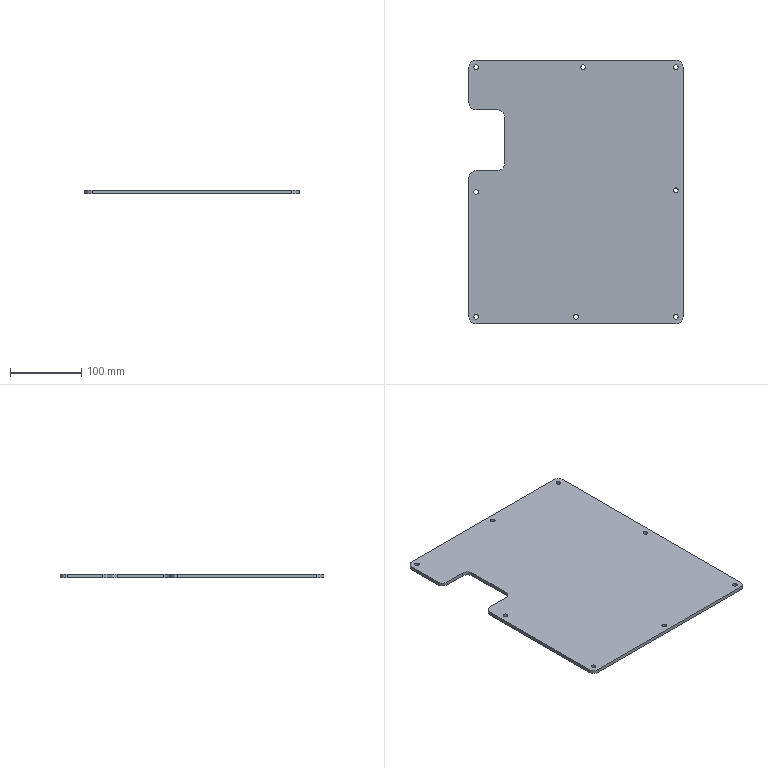Part | STEP file | 11-FG-01011 | 1 solid | 34 faces | box 300 x 370 x 5 mm | volume 531993 mm3 | cylinder 24 | plane 10 | commonest cylinder face diameters 6.5 x16 20 x8
STEP:
#1=CARTESIAN_POINT('',(-143.25,0.,0.));
#2=VERTEX_POINT('',#1);
#3=CARTESIAN_POINT('',(-136.75,0.,0.));
#4=VERTEX_POINT('',#3);
#5=CARTESIAN_POINT('',(-140.,0.,0.));
#6=DIRECTION('',(0.,0.,1.));
#7=DIRECTION('',(1.,0.,0.));
#8=AXIS2_PLACEMENT_3D('',#5,#6,#7);
#9=CIRCLE('',#8,3.25);
#10=EDGE_CURVE('',#2,#4,#9,.T.);
#11=ORIENTED_EDGE('',*,*,#10,.F.);
#12=CARTESIAN_POINT('',(-143.25,0.,5.));
#13=VERTEX_POINT('',#12);
#14=CARTESIAN_POINT('',(-143.25,0.,-5.));
#15=DIRECTION('',(0.,0.,1.));
#16=VECTOR('',#15,1000.);
#17=LINE('',#14,#16);
#18=EDGE_CURVE('',#2,#13,#17,.T.);
#19=ORIENTED_EDGE('',*,*,#18,.T.);
#20=CARTESIAN_POINT('',(-136.75,0.,5.));
#21=VERTEX_POINT('',#20);
#22=CARTESIAN_POINT('',(-140.,0.,5.));
#23=DIRECTION('',(0.,0.,1.));
#24=DIRECTION('',(1.,0.,0.));
#25=AXIS2_PLACEMENT_3D('',#22,#23,#24);
#26=CIRCLE('',#25,3.25);
#27=EDGE_CURVE('',#13,#21,#26,.T.);
#28=ORIENTED_EDGE('',*,*,#27,.T.);
#29=CARTESIAN_POINT('',(-136.75,0.,-5.));
#30=DIRECTION('',(0.,0.,1.));
#31=VECTOR('',#30,1000.);
#32=LINE('',#29,#31);
#33=EDGE_CURVE('',#4,#21,#32,.T.);
#34=ORIENTED_EDGE('',*,*,#33,.F.);
#35=EDGE_LOOP('',(#11,#19,#28,#34));
#36=FACE_OUTER_BOUND('',#35,.T.);
#37=CARTESIAN_POINT('',(-140.,0.,-5.));
#38=DIRECTION('',(0.,0.,1.));
#39=DIRECTION('',(1.,0.,0.));
#40=AXIS2_PLACEMENT_3D('',#37,#38,#39);
#41=CYLINDRICAL_SURFACE('',#40,3.25);
#42=ADVANCED_FACE('',(#36),#41,.F.);
#43=CARTESIAN_POINT('',(-143.25,-175.,0.));
#44=VERTEX_POINT('',#43);
#45=CARTESIAN_POINT('',(-136.75,-175.,0.));
#46=VERTEX_POINT('',#45);
#47=CARTESIAN_POINT('',(-140.,-175.,0.));
#48=DIRECTION('',(0.,0.,1.));
#49=DIRECTION('',(1.,0.,0.));
#50=AXIS2_PLACEMENT_3D('',#47,#48,#49);
#51=CIRCLE('',#50,3.25);
#52=EDGE_CURVE('',#44,#46,#51,.T.);
#53=ORIENTED_EDGE('',*,*,#52,.F.);
#54=CARTESIAN_POINT('',(-143.25,-175.,5.));
#55=VERTEX_POINT('',#54);
#56=CARTESIAN_POINT('',(-143.25,-175.,-5.));
#57=DIRECTION('',(0.,0.,1.));
#58=VECTOR('',#57,1000.);
#59=LINE('',#56,#58);
#60=EDGE_CURVE('',#44,#55,#59,.T.);
#61=ORIENTED_EDGE('',*,*,#60,.T.);
#62=CARTESIAN_POINT('',(-136.75,-175.,5.));
#63=VERTEX_POINT('',#62);
#64=CARTESIAN_POINT('',(-140.,-175.,5.));
#65=DIRECTION('',(0.,0.,1.));
#66=DIRECTION('',(1.,0.,0.));
#67=AXIS2_PLACEMENT_3D('',#64,#65,#66);
#68=CIRCLE('',#67,3.25);
#69=EDGE_CURVE('',#55,#63,#68,.T.);
#70=ORIENTED_EDGE('',*,*,#69,.T.);
#71=CARTESIAN_POINT('',(-136.75,-175.,-5.));
#72=DIRECTION('',(0.,0.,1.));
#73=VECTOR('',#72,1000.);
#74=LINE('',#71,#73);
#75=EDGE_CURVE('',#46,#63,#74,.T.);
#76=ORIENTED_EDGE('',*,*,#75,.F.);
#77=EDGE_LOOP('',(#53,#61,#70,#76));
#78=FACE_OUTER_BOUND('',#77,.T.);
#79=CARTESIAN_POINT('',(-140.,-175.,-5.));
#80=DIRECTION('',(0.,0.,1.));
#81=DIRECTION('',(1.,0.,0.));
#82=AXIS2_PLACEMENT_3D('',#79,#80,#81);
#83=CYLINDRICAL_SURFACE('',#82,3.25);
#84=ADVANCED_FACE('',(#78),#83,.F.);
#85=CARTESIAN_POINT('',(-3.25,-175.,0.));
#86=VERTEX_POINT('',#85);
#87=CARTESIAN_POINT('',(3.25,-175.,0.));
#88=VERTEX_POINT('',#87);
#89=CARTESIAN_POINT('',(0.,-175.,0.));
#90=DIRECTION('',(0.,0.,1.));
#91=DIRECTION('',(1.,0.,0.));
#92=AXIS2_PLACEMENT_3D('',#89,#90,#91);
#93=CIRCLE('',#92,3.25);
#94=EDGE_CURVE('',#86,#88,#93,.T.);
#95=ORIENTED_EDGE('',*,*,#94,.F.);
#96=CARTESIAN_POINT('',(-3.25,-175.,5.));
#97=VERTEX_POINT('',#96);
#98=CARTESIAN_POINT('',(-3.25,-175.,-5.));
#99=DIRECTION('',(0.,0.,1.));
#100=VECTOR('',#99,1000.);
#101=LINE('',#98,#100);
#102=EDGE_CURVE('',#86,#97,#101,.T.);
#103=ORIENTED_EDGE('',*,*,#102,.T.);
#104=CARTESIAN_POINT('',(3.25,-175.,5.));
#105=VERTEX_POINT('',#104);
#106=CARTESIAN_POINT('',(0.,-175.,5.));
#107=DIRECTION('',(0.,0.,1.));
#108=DIRECTION('',(1.,0.,0.));
#109=AXIS2_PLACEMENT_3D('',#106,#107,#108);
#110=CIRCLE('',#109,3.25);
#111=EDGE_CURVE('',#97,#105,#110,.T.);
#112=ORIENTED_EDGE('',*,*,#111,.T.);
#113=CARTESIAN_POINT('',(3.25,-175.,-5.));
#114=DIRECTION('',(0.,0.,1.));
#115=VECTOR('',#114,1000.);
#116=LINE('',#113,#115);
#117=EDGE_CURVE('',#88,#105,#116,.T.);
#118=ORIENTED_EDGE('',*,*,#117,.F.);
#119=EDGE_LOOP('',(#95,#103,#112,#118));
#120=FACE_OUTER_BOUND('',#119,.T.);
#121=CARTESIAN_POINT('',(0.,-175.,-5.));
#122=DIRECTION('',(0.,0.,1.));
#123=DIRECTION('',(1.,0.,0.));
#124=AXIS2_PLACEMENT_3D('',#121,#122,#123);
#125=CYLINDRICAL_SURFACE('',#124,3.25);
#126=ADVANCED_FACE('',(#120),#125,.F.);
#127=CARTESIAN_POINT('',(136.75,-175.,0.));
#128=VERTEX_POINT('',#127);
#129=CARTESIAN_POINT('',(143.25,-175.,0.));
#130=VERTEX_POINT('',#129);
#131=CARTESIAN_POINT('',(140.,-175.,0.));
#132=DIRECTION('',(0.,0.,1.));
#133=DIRECTION('',(1.,0.,0.));
#134=AXIS2_PLACEMENT_3D('',#131,#132,#133);
#135=CIRCLE('',#134,3.25);
#136=EDGE_CURVE('',#128,#130,#135,.T.);
#137=ORIENTED_EDGE('',*,*,#136,.F.);
#138=CARTESIAN_POINT('',(136.75,-175.,5.));
#139=VERTEX_POINT('',#138);
#140=CARTESIAN_POINT('',(136.75,-175.,-5.));
#141=DIRECTION('',(0.,0.,1.));
#142=VECTOR('',#141,1000.);
#143=LINE('',#140,#142);
#144=EDGE_CURVE('',#128,#139,#143,.T.);
#145=ORIENTED_EDGE('',*,*,#144,.T.);
#146=CARTESIAN_POINT('',(143.25,-175.,5.));
#147=VERTEX_POINT('',#146);
#148=CARTESIAN_POINT('',(140.,-175.,5.));
#149=DIRECTION('',(0.,0.,1.));
#150=DIRECTION('',(1.,0.,0.));
#151=AXIS2_PLACEMENT_3D('',#148,#149,#150);
#152=CIRCLE('',#151,3.25);
#153=EDGE_CURVE('',#139,#147,#152,.T.);
#154=ORIENTED_EDGE('',*,*,#153,.T.);
#155=CARTESIAN_POINT('',(143.25,-175.,-5.));
#156=DIRECTION('',(0.,0.,1.));
#157=VECTOR('',#156,1000.);
#158=LINE('',#155,#157);
#159=EDGE_CURVE('',#130,#147,#158,.T.);
#160=ORIENTED_EDGE('',*,*,#159,.F.);
#161=EDGE_LOOP('',(#137,#145,#154,#160));
#162=FACE_OUTER_BOUND('',#161,.T.);
#163=CARTESIAN_POINT('',(140.,-175.,-5.));
#164=DIRECTION('',(0.,0.,1.));
#165=DIRECTION('',(1.,0.,0.));
#166=AXIS2_PLACEMENT_3D('',#163,#164,#165);
#167=CYLINDRICAL_SURFACE('',#166,3.25);
#168=ADVANCED_FACE('',(#162),#167,.F.);
#169=CARTESIAN_POINT('',(136.75,2.5,0.));
#170=VERTEX_POINT('',#169);
#171=CARTESIAN_POINT('',(143.25,2.5,0.));
#172=VERTEX_POINT('',#171);
#173=CARTESIAN_POINT('',(140.,2.5,0.));
#174=DIRECTION('',(0.,0.,1.));
#175=DIRECTION('',(1.,0.,0.));
#176=AXIS2_PLACEMENT_3D('',#173,#174,#175);
#177=CIRCLE('',#176,3.25);
#178=EDGE_CURVE('',#170,#172,#177,.T.);
#179=ORIENTED_EDGE('',*,*,#178,.F.);
#180=CARTESIAN_POINT('',(136.75,2.5,5.));
#181=VERTEX_POINT('',#180);
#182=CARTESIAN_POINT('',(136.75,2.5,-5.));
#183=DIRECTION('',(0.,0.,1.));
#184=VECTOR('',#183,1000.);
#185=LINE('',#182,#184);
#186=EDGE_CURVE('',#170,#181,#185,.T.);
#187=ORIENTED_EDGE('',*,*,#186,.T.);
#188=CARTESIAN_POINT('',(143.25,2.5,5.));
#189=VERTEX_POINT('',#188);
#190=CARTESIAN_POINT('',(140.,2.5,5.));
#191=DIRECTION('',(0.,0.,1.));
#192=DIRECTION('',(1.,0.,0.));
#193=AXIS2_PLACEMENT_3D('',#190,#191,#192);
#194=CIRCLE('',#193,3.25);
#195=EDGE_CURVE('',#181,#189,#194,.T.);
#196=ORIENTED_EDGE('',*,*,#195,.T.);
#197=CARTESIAN_POINT('',(143.25,2.5,-5.));
#198=DIRECTION('',(0.,0.,1.));
#199=VECTOR('',#198,1000.);
#200=LINE('',#197,#199);
#201=EDGE_CURVE('',#172,#189,#200,.T.);
#202=ORIENTED_EDGE('',*,*,#201,.F.);
#203=EDGE_LOOP('',(#179,#187,#196,#202));
#204=FACE_OUTER_BOUND('',#203,.T.);
#205=CARTESIAN_POINT('',(140.,2.5,-5.));
#206=DIRECTION('',(0.,0.,1.));
#207=DIRECTION('',(1.,0.,0.));
#208=AXIS2_PLACEMENT_3D('',#205,#206,#207);
#209=CYLINDRICAL_SURFACE('',#208,3.25);
#210=ADVANCED_FACE('',(#204),#209,.F.);
#211=CARTESIAN_POINT('',(136.75,175.,0.));
#212=VERTEX_POINT('',#211);
#213=CARTESIAN_POINT('',(143.25,175.,0.));
#214=VERTEX_POINT('',#213);
#215=CARTESIAN_POINT('',(140.,175.,0.));
#216=DIRECTION('',(0.,0.,1.));
#217=DIRECTION('',(1.,0.,0.));
#218=AXIS2_PLACEMENT_3D('',#215,#216,#217);
#219=CIRCLE('',#218,3.25);
#220=EDGE_CURVE('',#212,#214,#219,.T.);
#221=ORIENTED_EDGE('',*,*,#220,.F.);
#222=CARTESIAN_POINT('',(136.75,175.,5.));
#223=VERTEX_POINT('',#222);
#224=CARTESIAN_POINT('',(136.75,175.,-5.));
#225=DIRECTION('',(0.,0.,1.));
#226=VECTOR('',#225,1000.);
#227=LINE('',#224,#226);
#228=EDGE_CURVE('',#212,#223,#227,.T.);
#229=ORIENTED_EDGE('',*,*,#228,.T.);
#230=CARTESIAN_POINT('',(143.25,175.,5.));
#231=VERTEX_POINT('',#230);
#232=CARTESIAN_POINT('',(140.,175.,5.));
#233=DIRECTION('',(0.,0.,1.));
#234=DIRECTION('',(1.,0.,0.));
#235=AXIS2_PLACEMENT_3D('',#232,#233,#234);
#236=CIRCLE('',#235,3.25);
#237=EDGE_CURVE('',#223,#231,#236,.T.);
#238=ORIENTED_EDGE('',*,*,#237,.T.);
#239=CARTESIAN_POINT('',(143.25,175.,-5.));
#240=DIRECTION('',(0.,0.,1.));
#241=VECTOR('',#240,1000.);
#242=LINE('',#239,#241);
#243=EDGE_CURVE('',#214,#231,#242,.T.);
#244=ORIENTED_EDGE('',*,*,#243,.F.);
#245=EDGE_LOOP('',(#221,#229,#238,#244));
#246=FACE_OUTER_BOUND('',#245,.T.);
#247=CARTESIAN_POINT('',(140.,175.,-5.));
#248=DIRECTION('',(0.,0.,1.));
#249=DIRECTION('',(1.,0.,0.));
#250=AXIS2_PLACEMENT_3D('',#247,#248,#249);
#251=CYLINDRICAL_SURFACE('',#250,3.25);
#252=ADVANCED_FACE('',(#246),#251,.F.);
#253=CARTESIAN_POINT('',(6.75,175.,0.));
#254=VERTEX_POINT('',#253);
#255=CARTESIAN_POINT('',(13.25,175.,0.));
#256=VERTEX_POINT('',#255);
#257=CARTESIAN_POINT('',(10.,175.,0.));
#258=DIRECTION('',(0.,0.,1.));
#259=DIRECTION('',(1.,0.,0.));
#260=AXIS2_PLACEMENT_3D('',#257,#258,#259);
#261=CIRCLE('',#260,3.25);
#262=EDGE_CURVE('',#254,#256,#261,.T.);
#263=ORIENTED_EDGE('',*,*,#262,.F.);
#264=CARTESIAN_POINT('',(6.75,175.,5.));
#265=VERTEX_POINT('',#264);
#266=CARTESIAN_POINT('',(6.75,175.,-5.));
#267=DIRECTION('',(0.,0.,1.));
#268=VECTOR('',#267,1000.);
#269=LINE('',#266,#268);
#270=EDGE_CURVE('',#254,#265,#269,.T.);
#271=ORIENTED_EDGE('',*,*,#270,.T.);
#272=CARTESIAN_POINT('',(13.25,175.,5.));
#273=VERTEX_POINT('',#272);
#274=CARTESIAN_POINT('',(10.,175.,5.));
#275=DIRECTION('',(0.,0.,1.));
#276=DIRECTION('',(1.,0.,0.));
#277=AXIS2_PLACEMENT_3D('',#274,#275,#276);
#278=CIRCLE('',#277,3.25);
#279=EDGE_CURVE('',#265,#273,#278,.T.);
#280=ORIENTED_EDGE('',*,*,#279,.T.);
#281=CARTESIAN_POINT('',(13.25,175.,-5.));
#282=DIRECTION('',(0.,0.,1.));
#283=VECTOR('',#282,1000.);
#284=LINE('',#281,#283);
#285=EDGE_CURVE('',#256,#273,#284,.T.);
#286=ORIENTED_EDGE('',*,*,#285,.F.);
#287=EDGE_LOOP('',(#263,#271,#280,#286));
#288=FACE_OUTER_BOUND('',#287,.T.);
#289=CARTESIAN_POINT('',(10.,175.,-5.));
#290=DIRECTION('',(0.,0.,1.));
#291=DIRECTION('',(1.,0.,0.));
#292=AXIS2_PLACEMENT_3D('',#289,#290,#291);
#293=CYLINDRICAL_SURFACE('',#292,3.25);
#294=ADVANCED_FACE('',(#288),#293,.F.);
#295=CARTESIAN_POINT('',(-143.25,175.,0.));
#296=VERTEX_POINT('',#295);
#297=CARTESIAN_POINT('',(-136.75,175.,0.));
#298=VERTEX_POINT('',#297);
#299=CARTESIAN_POINT('',(-140.,175.,0.));
#300=DIRECTION('',(0.,0.,1.));
#301=DIRECTION('',(1.,0.,0.));
#302=AXIS2_PLACEMENT_3D('',#299,#300,#301);
#303=CIRCLE('',#302,3.25);
#304=EDGE_CURVE('',#296,#298,#303,.T.);
#305=ORIENTED_EDGE('',*,*,#304,.F.);
#306=CARTESIAN_POINT('',(-143.25,175.,5.));
#307=VERTEX_POINT('',#306);
#308=CARTESIAN_POINT('',(-143.25,175.,-5.));
#309=DIRECTION('',(0.,0.,1.));
#310=VECTOR('',#309,1000.);
#311=LINE('',#308,#310);
#312=EDGE_CURVE('',#296,#307,#311,.T.);
#313=ORIENTED_EDGE('',*,*,#312,.T.);
#314=CARTESIAN_POINT('',(-136.75,175.,5.));
#315=VERTEX_POINT('',#314);
#316=CARTESIAN_POINT('',(-140.,175.,5.));
#317=DIRECTION('',(0.,0.,1.));
#318=DIRECTION('',(1.,0.,0.));
#319=AXIS2_PLACEMENT_3D('',#316,#317,#318);
#320=CIRCLE('',#319,3.25);
#321=EDGE_CURVE('',#307,#315,#320,.T.);
#322=ORIENTED_EDGE('',*,*,#321,.T.);
#323=CARTESIAN_POINT('',(-136.75,175.,-5.));
#324=DIRECTION('',(0.,0.,1.));
#325=VECTOR('',#324,1000.);
#326=LINE('',#323,#325);
#327=EDGE_CURVE('',#298,#315,#326,.T.);
#328=ORIENTED_EDGE('',*,*,#327,.F.);
#329=EDGE_LOOP('',(#305,#313,#322,#328));
#330=FACE_OUTER_BOUND('',#329,.T.);
#331=CARTESIAN_POINT('',(-140.,175.,-5.));
#332=DIRECTION('',(0.,0.,1.));
#333=DIRECTION('',(1.,0.,0.));
#334=AXIS2_PLACEMENT_3D('',#331,#332,#333);
#335=CYLINDRICAL_SURFACE('',#334,3.25);
#336=ADVANCED_FACE('',(#330),#335,.F.);
#337=CARTESIAN_POINT('',(-150.,175.,0.));
#338=VERTEX_POINT('',#337);
#339=CARTESIAN_POINT('',(-150.,125.,0.));
#340=VERTEX_POINT('',#339);
#341=CARTESIAN_POINT('',(-150.,185.,0.));
#342=DIRECTION('',(0.,-1.,0.));
#343=VECTOR('',#342,1000.);
#344=LINE('',#341,#343);
#345=EDGE_CURVE('',#338,#340,#344,.T.);
#346=ORIENTED_EDGE('',*,*,#345,.T.);
#347=CARTESIAN_POINT('',(-150.,125.,5.));
#348=VERTEX_POINT('',#347);
#349=CARTESIAN_POINT('',(-150.,125.,5.));
#350=DIRECTION('',(0.,0.,1.));
#351=VECTOR('',#350,1000.);
#352=LINE('',#349,#351);
#353=EDGE_CURVE('',#340,#348,#352,.T.);
#354=ORIENTED_EDGE('',*,*,#353,.T.);
#355=CARTESIAN_POINT('',(-150.,175.,5.));
#356=VERTEX_POINT('',#355);
#357=CARTESIAN_POINT('',(-150.,185.,5.));
#358=DIRECTION('',(0.,-1.,0.));
#359=VECTOR('',#358,1000.);
#360=LINE('',#357,#359);
#361=EDGE_CURVE('',#356,#348,#360,.T.);
#362=ORIENTED_EDGE('',*,*,#361,.F.);
#363=CARTESIAN_POINT('',(-150.,175.,5.));
#364=DIRECTION('',(0.,0.,-1.));
#365=VECTOR('',#364,1000.);
#366=LINE('',#363,#365);
#367=EDGE_CURVE('',#356,#338,#366,.T.);
#368=ORIENTED_EDGE('',*,*,#367,.T.);
#369=EDGE_LOOP('',(#346,#354,#362,#368));
#370=FACE_OUTER_BOUND('',#369,.T.);
#371=CARTESIAN_POINT('',(-150.,185.,5.));
#372=DIRECTION('',(1.,0.,0.));
#373=DIRECTION('',(0.,1.,0.));
#374=AXIS2_PLACEMENT_3D('',#371,#372,#373);
#375=PLANE('',#374);
#376=ADVANCED_FACE('',(#370),#375,.F.);
#377=CARTESIAN_POINT('',(150.,-175.,5.));
#378=VERTEX_POINT('',#377);
#379=CARTESIAN_POINT('',(150.,175.,5.));
#380=VERTEX_POINT('',#379);
#381=CARTESIAN_POINT('',(150.,185.,5.));
#382=DIRECTION('',(0.,1.,0.));
#383=VECTOR('',#382,1000.);
#384=LINE('',#381,#383);
#385=EDGE_CURVE('',#378,#380,#384,.T.);
#386=ORIENTED_EDGE('',*,*,#385,.F.);
#387=CARTESIAN_POINT('',(150.,-175.,0.));
#388=VERTEX_POINT('',#387);
#389=CARTESIAN_POINT('',(150.,-175.,5.));
#390=DIRECTION('',(0.,0.,-1.));
#391=VECTOR('',#390,1000.);
#392=LINE('',#389,#391);
#393=EDGE_CURVE('',#378,#388,#392,.T.);
#394=ORIENTED_EDGE('',*,*,#393,.T.);
#395=CARTESIAN_POINT('',(150.,175.,0.));
#396=VERTEX_POINT('',#395);
#397=CARTESIAN_POINT('',(150.,185.,0.));
#398=DIRECTION('',(0.,1.,0.));
#399=VECTOR('',#398,1000.);
#400=LINE('',#397,#399);
#401=EDGE_CURVE('',#388,#396,#400,.T.);
#402=ORIENTED_EDGE('',*,*,#401,.T.);
#403=CARTESIAN_POINT('',(150.,175.,5.));
#404=DIRECTION('',(0.,0.,1.));
#405=VECTOR('',#404,1000.);
#406=LINE('',#403,#405);
#407=EDGE_CURVE('',#396,#380,#406,.T.);
#408=ORIENTED_EDGE('',*,*,#407,.T.);
#409=EDGE_LOOP('',(#386,#394,#402,#408));
#410=FACE_OUTER_BOUND('',#409,.T.);
#411=CARTESIAN_POINT('',(150.,185.,5.));
#412=DIRECTION('',(-1.,0.,0.));
#413=DIRECTION('',(0.,-1.,0.));
#414=AXIS2_PLACEMENT_3D('',#411,#412,#413);
#415=PLANE('',#414);
#416=ADVANCED_FACE('',(#410),#415,.F.);
#417=CARTESIAN_POINT('',(140.,185.,5.));
#418=VERTEX_POINT('',#417);
#419=CARTESIAN_POINT('',(-140.,185.,5.));
#420=VERTEX_POINT('',#419);
#421=CARTESIAN_POINT('',(-150.,185.,5.));
#422=DIRECTION('',(-1.,0.,0.));
#423=VECTOR('',#422,1000.);
#424=LINE('',#421,#423);
#425=EDGE_CURVE('',#418,#420,#424,.T.);
#426=ORIENTED_EDGE('',*,*,#425,.F.);
#427=CARTESIAN_POINT('',(140.,185.,0.));
#428=VERTEX_POINT('',#427);
#429=CARTESIAN_POINT('',(140.,185.,5.));
#430=DIRECTION('',(0.,0.,-1.));
#431=VECTOR('',#430,1000.);
#432=LINE('',#429,#431);
#433=EDGE_CURVE('',#418,#428,#432,.T.);
#434=ORIENTED_EDGE('',*,*,#433,.T.);
#435=CARTESIAN_POINT('',(-140.,185.,0.));
#436=VERTEX_POINT('',#435);
#437=CARTESIAN_POINT('',(-150.,185.,0.));
#438=DIRECTION('',(-1.,0.,0.));
#439=VECTOR('',#438,1000.);
#440=LINE('',#437,#439);
#441=EDGE_CURVE('',#428,#436,#440,.T.);
#442=ORIENTED_EDGE('',*,*,#441,.T.);
#443=CARTESIAN_POINT('',(-140.,185.,5.));
#444=DIRECTION('',(0.,0.,1.));
#445=VECTOR('',#444,1000.);
#446=LINE('',#443,#445);
#447=EDGE_CURVE('',#436,#420,#446,.T.);
#448=ORIENTED_EDGE('',*,*,#447,.T.);
#449=EDGE_LOOP('',(#426,#434,#442,#448));
#450=FACE_OUTER_BOUND('',#449,.T.);
#451=CARTESIAN_POINT('',(-150.,185.,5.));
#452=DIRECTION('',(0.,-1.,0.));
#453=DIRECTION('',(0.,0.,-1.));
#454=AXIS2_PLACEMENT_3D('',#451,#452,#453);
#455=PLANE('',#454);
#456=ADVANCED_FACE('',(#450),#455,.F.);
#457=CARTESIAN_POINT('',(-150.,20.,5.));
#458=VERTEX_POINT('',#457);
#459=CARTESIAN_POINT('',(-150.,-175.,5.));
#460=VERTEX_POINT('',#459);
#461=CARTESIAN_POINT('',(-150.,185.,5.));
#462=DIRECTION('',(0.,-1.,0.));
#463=VECTOR('',#462,1000.);
#464=LINE('',#461,#463);
#465=EDGE_CURVE('',#458,#460,#464,.T.);
#466=ORIENTED_EDGE('',*,*,#465,.F.);
#467=CARTESIAN_POINT('',(-150.,20.,0.));
#468=VERTEX_POINT('',#467);
#469=CARTESIAN_POINT('',(-150.,20.,5.));
#470=DIRECTION('',(0.,0.,-1.));
#471=VECTOR('',#470,1000.);
#472=LINE('',#469,#471);
#473=EDGE_CURVE('',#458,#468,#472,.T.);
#474=ORIENTED_EDGE('',*,*,#473,.T.);
#475=CARTESIAN_POINT('',(-150.,-175.,0.));
#476=VERTEX_POINT('',#475);
#477=CARTESIAN_POINT('',(-150.,185.,0.));
#478=DIRECTION('',(0.,-1.,0.));
#479=VECTOR('',#478,1000.);
#480=LINE('',#477,#479);
#481=EDGE_CURVE('',#468,#476,#480,.T.);
#482=ORIENTED_EDGE('',*,*,#481,.T.);
#483=CARTESIAN_POINT('',(-150.,-175.,5.));
#484=DIRECTION('',(0.,0.,1.));
#485=VECTOR('',#484,1000.);
#486=LINE('',#483,#485);
#487=EDGE_CURVE('',#476,#460,#486,.T.);
#488=ORIENTED_EDGE('',*,*,#487,.T.);
#489=EDGE_LOOP('',(#466,#474,#482,#488));
#490=FACE_OUTER_BOUND('',#489,.T.);
#491=CARTESIAN_POINT('',(-150.,185.,5.));
#492=DIRECTION('',(1.,0.,0.));
#493=DIRECTION('',(0.,1.,0.));
#494=AXIS2_PLACEMENT_3D('',#491,#492,#493);
#495=PLANE('',#494);
#496=ADVANCED_FACE('',(#490),#495,.F.);
#497=CARTESIAN_POINT('',(-140.,-185.,5.));
#498=VERTEX_POINT('',#497);
#499=CARTESIAN_POINT('',(140.,-185.,5.));
#500=VERTEX_POINT('',#499);
#501=CARTESIAN_POINT('',(-150.,-185.,5.));
#502=DIRECTION('',(1.,0.,0.));
#503=VECTOR('',#502,1000.);
#504=LINE('',#501,#503);
#505=EDGE_CURVE('',#498,#500,#504,.T.);
#506=ORIENTED_EDGE('',*,*,#505,.F.);
#507=CARTESIAN_POINT('',(-140.,-185.,0.));
#508=VERTEX_POINT('',#507);
#509=CARTESIAN_POINT('',(-140.,-185.,5.));
#510=DIRECTION('',(0.,0.,-1.));
#511=VECTOR('',#510,1000.);
#512=LINE('',#509,#511);
#513=EDGE_CURVE('',#498,#508,#512,.T.);
#514=ORIENTED_EDGE('',*,*,#513,.T.);
#515=CARTESIAN_POINT('',(140.,-185.,0.));
#516=VERTEX_POINT('',#515);
#517=CARTESIAN_POINT('',(-150.,-185.,0.));
#518=DIRECTION('',(1.,0.,0.));
#519=VECTOR('',#518,1000.);
#520=LINE('',#517,#519);
#521=EDGE_CURVE('',#508,#516,#520,.T.);
#522=ORIENTED_EDGE('',*,*,#521,.T.);
#523=CARTESIAN_POINT('',(140.,-185.,5.));
#524=DIRECTION('',(0.,0.,1.));
#525=VECTOR('',#524,1000.);
#526=LINE('',#523,#525);
#527=EDGE_CURVE('',#516,#500,#526,.T.);
#528=ORIENTED_EDGE('',*,*,#527,.T.);
#529=EDGE_LOOP('',(#506,#514,#522,#528));
#530=FACE_OUTER_BOUND('',#529,.T.);
#531=CARTESIAN_POINT('',(-150.,-185.,5.));
#532=DIRECTION('',(0.,1.,0.));
#533=DIRECTION('',(0.,0.,1.));
#534=AXIS2_PLACEMENT_3D('',#531,#532,#533);
#535=PLANE('',#534);
#536=ADVANCED_FACE('',(#530),#535,.F.);
#537=CARTESIAN_POINT('',(-140.,0.,5.));
#538=DIRECTION('',(0.,0.,1.));
#539=DIRECTION('',(1.,0.,0.));
#540=AXIS2_PLACEMENT_3D('',#537,#538,#539);
#541=CIRCLE('',#540,3.25);
#542=EDGE_CURVE('',#21,#13,#541,.T.);
#543=ORIENTED_EDGE('',*,*,#542,.F.);
#544=ORIENTED_EDGE('',*,*,#27,.F.);
#545=EDGE_LOOP('',(#543,#544));
#546=FACE_BOUND('',#545,.T.);
#547=CARTESIAN_POINT('',(-140.,-175.,5.));
#548=DIRECTION('',(0.,0.,1.));
#549=DIRECTION('',(1.,0.,0.));
#550=AXIS2_PLACEMENT_3D('',#547,#548,#549);
#551=CIRCLE('',#550,3.25);
#552=EDGE_CURVE('',#63,#55,#551,.T.);
#553=ORIENTED_EDGE('',*,*,#552,.F.);
#554=ORIENTED_EDGE('',*,*,#69,.F.);
#555=EDGE_LOOP('',(#553,#554));
#556=FACE_BOUND('',#555,.T.);
#557=CARTESIAN_POINT('',(0.,-175.,5.));
#558=DIRECTION('',(0.,0.,1.));
#559=DIRECTION('',(1.,0.,0.));
#560=AXIS2_PLACEMENT_3D('',#557,#558,#559);
#561=CIRCLE('',#560,3.25);
#562=EDGE_CURVE('',#105,#97,#561,.T.);
#563=ORIENTED_EDGE('',*,*,#562,.F.);
#564=ORIENTED_EDGE('',*,*,#111,.F.);
#565=EDGE_LOOP('',(#563,#564));
#566=FACE_BOUND('',#565,.T.);
#567=CARTESIAN_POINT('',(140.,-175.,5.));
#568=DIRECTION('',(0.,0.,1.));
#569=DIRECTION('',(1.,0.,0.));
#570=AXIS2_PLACEMENT_3D('',#567,#568,#569);
#571=CIRCLE('',#570,3.25);
#572=EDGE_CURVE('',#147,#139,#571,.T.);
#573=ORIENTED_EDGE('',*,*,#572,.F.);
#574=ORIENTED_EDGE('',*,*,#153,.F.);
#575=EDGE_LOOP('',(#573,#574));
#576=FACE_BOUND('',#575,.T.);
#577=CARTESIAN_POINT('',(140.,2.5,5.));
#578=DIRECTION('',(0.,0.,1.));
#579=DIRECTION('',(1.,0.,0.));
#580=AXIS2_PLACEMENT_3D('',#577,#578,#579);
#581=CIRCLE('',#580,3.25);
#582=EDGE_CURVE('',#189,#181,#581,.T.);
#583=ORIENTED_EDGE('',*,*,#582,.F.);
#584=ORIENTED_EDGE('',*,*,#195,.F.);
#585=EDGE_LOOP('',(#583,#584));
#586=FACE_BOUND('',#585,.T.);
#587=CARTESIAN_POINT('',(140.,175.,5.));
#588=DIRECTION('',(0.,0.,1.));
#589=DIRECTION('',(1.,0.,0.));
#590=AXIS2_PLACEMENT_3D('',#587,#588,#589);
#591=CIRCLE('',#590,3.25);
#592=EDGE_CURVE('',#231,#223,#591,.T.);
#593=ORIENTED_EDGE('',*,*,#592,.F.);
#594=ORIENTED_EDGE('',*,*,#237,.F.);
#595=EDGE_LOOP('',(#593,#594));
#596=FACE_BOUND('',#595,.T.);
#597=CARTESIAN_POINT('',(10.,175.,5.));
#598=DIRECTION('',(0.,0.,1.));
#599=DIRECTION('',(1.,0.,0.));
#600=AXIS2_PLACEMENT_3D('',#597,#598,#599);
#601=CIRCLE('',#600,3.25);
#602=EDGE_CURVE('',#273,#265,#601,.T.);
#603=ORIENTED_EDGE('',*,*,#602,.F.);
#604=ORIENTED_EDGE('',*,*,#279,.F.);
#605=EDGE_LOOP('',(#603,#604));
#606=FACE_BOUND('',#605,.T.);
#607=CARTESIAN_POINT('',(-140.,175.,5.));
#608=DIRECTION('',(0.,0.,1.));
#609=DIRECTION('',(1.,0.,0.));
#610=AXIS2_PLACEMENT_3D('',#607,#608,#609);
#611=CIRCLE('',#610,3.25);
#612=EDGE_CURVE('',#315,#307,#611,.T.);
#613=ORIENTED_EDGE('',*,*,#612,.F.);
#614=ORIENTED_EDGE('',*,*,#321,.F.);
#615=EDGE_LOOP('',(#613,#614));
#616=FACE_BOUND('',#615,.T.);
#617=ORIENTED_EDGE('',*,*,#361,.T.);
#618=CARTESIAN_POINT('',(-140.,115.,5.));
#619=VERTEX_POINT('',#618);
#620=CARTESIAN_POINT('',(-140.,125.,5.));
#621=DIRECTION('',(0.,0.,1.));
#622=DIRECTION('',(1.,0.,0.));
#623=AXIS2_PLACEMENT_3D('',#620,#621,#622);
#624=CIRCLE('',#623,10.);
#625=EDGE_CURVE('',#348,#619,#624,.T.);
#626=ORIENTED_EDGE('',*,*,#625,.T.);
#627=CARTESIAN_POINT('',(-110.,115.,5.));
#628=VERTEX_POINT('',#627);
#629=CARTESIAN_POINT('',(-100.,115.,5.));
#630=DIRECTION('',(-1.,0.,0.));
#631=VECTOR('',#630,1000.);
#632=LINE('',#629,#631);
#633=EDGE_CURVE('',#628,#619,#632,.T.);
#634=ORIENTED_EDGE('',*,*,#633,.F.);
#635=CARTESIAN_POINT('',(-100.,105.,5.));
#636=VERTEX_POINT('',#635);
#637=CARTESIAN_POINT('',(-110.,105.,5.));
#638=DIRECTION('',(0.,0.,-1.));
#639=DIRECTION('',(1.,0.,0.));
#640=AXIS2_PLACEMENT_3D('',#637,#638,#639);
#641=CIRCLE('',#640,10.);
#642=EDGE_CURVE('',#628,#636,#641,.T.);
#643=ORIENTED_EDGE('',*,*,#642,.T.);
#644=CARTESIAN_POINT('',(-100.,40.,5.));
#645=VERTEX_POINT('',#644);
#646=CARTESIAN_POINT('',(-100.,30.,5.));
#647=DIRECTION('',(0.,1.,0.));
#648=VECTOR('',#647,1000.);
#649=LINE('',#646,#648);
#650=EDGE_CURVE('',#645,#636,#649,.T.);
#651=ORIENTED_EDGE('',*,*,#650,.F.);
#652=CARTESIAN_POINT('',(-110.,30.,5.));
#653=VERTEX_POINT('',#652);
#654=CARTESIAN_POINT('',(-110.,40.,5.));
#655=DIRECTION('',(0.,0.,-1.));
#656=DIRECTION('',(1.,0.,0.));
#657=AXIS2_PLACEMENT_3D('',#654,#655,#656);
#658=CIRCLE('',#657,10.);
#659=EDGE_CURVE('',#645,#653,#658,.T.);
#660=ORIENTED_EDGE('',*,*,#659,.T.);
#661=CARTESIAN_POINT('',(-140.,30.,5.));
#662=VERTEX_POINT('',#661);
#663=CARTESIAN_POINT('',(-100.,30.,5.));
#664=DIRECTION('',(1.,0.,0.));
#665=VECTOR('',#664,1000.);
#666=LINE('',#663,#665);
#667=EDGE_CURVE('',#662,#653,#666,.T.);
#668=ORIENTED_EDGE('',*,*,#667,.F.);
#669=CARTESIAN_POINT('',(-140.,20.,5.));
#670=DIRECTION('',(0.,0.,1.));
#671=DIRECTION('',(1.,0.,0.));
#672=AXIS2_PLACEMENT_3D('',#669,#670,#671);
#673=CIRCLE('',#672,10.);
#674=EDGE_CURVE('',#662,#458,#673,.T.);
#675=ORIENTED_EDGE('',*,*,#674,.T.);
#676=ORIENTED_EDGE('',*,*,#465,.T.);
#677=CARTESIAN_POINT('',(-140.,-175.,5.));
#678=DIRECTION('',(0.,0.,1.));
#679=DIRECTION('',(1.,0.,0.));
#680=AXIS2_PLACEMENT_3D('',#677,#678,#679);
#681=CIRCLE('',#680,10.);
#682=EDGE_CURVE('',#460,#498,#681,.T.);
#683=ORIENTED_EDGE('',*,*,#682,.T.);
#684=ORIENTED_EDGE('',*,*,#505,.T.);
#685=CARTESIAN_POINT('',(140.,-175.,5.));
#686=DIRECTION('',(0.,0.,1.));
#687=DIRECTION('',(1.,0.,0.));
#688=AXIS2_PLACEMENT_3D('',#685,#686,#687);
#689=CIRCLE('',#688,10.);
#690=EDGE_CURVE('',#500,#378,#689,.T.);
#691=ORIENTED_EDGE('',*,*,#690,.T.);
#692=ORIENTED_EDGE('',*,*,#385,.T.);
#693=CARTESIAN_POINT('',(140.,175.,5.));
#694=DIRECTION('',(0.,0.,1.));
#695=DIRECTION('',(1.,0.,0.));
#696=AXIS2_PLACEMENT_3D('',#693,#694,#695);
#697=CIRCLE('',#696,10.);
#698=EDGE_CURVE('',#380,#418,#697,.T.);
#699=ORIENTED_EDGE('',*,*,#698,.T.);
#700=ORIENTED_EDGE('',*,*,#425,.T.);
#701=CARTESIAN_POINT('',(-140.,175.,5.));
#702=DIRECTION('',(0.,0.,1.));
#703=DIRECTION('',(1.,0.,0.));
#704=AXIS2_PLACEMENT_3D('',#701,#702,#703);
#705=CIRCLE('',#704,10.);
#706=EDGE_CURVE('',#420,#356,#705,.T.);
#707=ORIENTED_EDGE('',*,*,#706,.T.);
#708=EDGE_LOOP('',(#617,#626,#634,#643,#651,#660,#668,#675,#676,#683,#684,#691,#692,#699,#700,#707));
#709=FACE_OUTER_BOUND('',#708,.T.);
#710=CARTESIAN_POINT('',(0.,0.,5.));
#711=DIRECTION('',(0.,0.,1.));
#712=DIRECTION('',(1.,0.,0.));
#713=AXIS2_PLACEMENT_3D('',#710,#711,#712);
#714=PLANE('',#713);
#715=ADVANCED_FACE('',(#546,#556,#566,#576,#586,#596,#606,#616,#709),#714,.T.);
#716=CARTESIAN_POINT('',(-140.,0.,0.));
#717=DIRECTION('',(0.,0.,1.));
#718=DIRECTION('',(1.,0.,0.));
#719=AXIS2_PLACEMENT_3D('',#716,#717,#718);
#720=CIRCLE('',#719,3.25);
#721=EDGE_CURVE('',#4,#2,#720,.T.);
#722=ORIENTED_EDGE('',*,*,#721,.T.);
#723=ORIENTED_EDGE('',*,*,#10,.T.);
#724=EDGE_LOOP('',(#722,#723));
#725=FACE_BOUND('',#724,.T.);
#726=CARTESIAN_POINT('',(-140.,-175.,0.));
#727=DIRECTION('',(0.,0.,1.));
#728=DIRECTION('',(1.,0.,0.));
#729=AXIS2_PLACEMENT_3D('',#726,#727,#728);
#730=CIRCLE('',#729,3.25);
#731=EDGE_CURVE('',#46,#44,#730,.T.);
#732=ORIENTED_EDGE('',*,*,#731,.T.);
#733=ORIENTED_EDGE('',*,*,#52,.T.);
#734=EDGE_LOOP('',(#732,#733));
#735=FACE_BOUND('',#734,.T.);
#736=CARTESIAN_POINT('',(0.,-175.,0.));
#737=DIRECTION('',(0.,0.,1.));
#738=DIRECTION('',(1.,0.,0.));
#739=AXIS2_PLACEMENT_3D('',#736,#737,#738);
#740=CIRCLE('',#739,3.25);
#741=EDGE_CURVE('',#88,#86,#740,.T.);
#742=ORIENTED_EDGE('',*,*,#741,.T.);
#743=ORIENTED_EDGE('',*,*,#94,.T.);
#744=EDGE_LOOP('',(#742,#743));
#745=FACE_BOUND('',#744,.T.);
#746=CARTESIAN_POINT('',(140.,-175.,0.));
#747=DIRECTION('',(0.,0.,1.));
#748=DIRECTION('',(1.,0.,0.));
#749=AXIS2_PLACEMENT_3D('',#746,#747,#748);
#750=CIRCLE('',#749,3.25);
#751=EDGE_CURVE('',#130,#128,#750,.T.);
#752=ORIENTED_EDGE('',*,*,#751,.T.);
#753=ORIENTED_EDGE('',*,*,#136,.T.);
#754=EDGE_LOOP('',(#752,#753));
#755=FACE_BOUND('',#754,.T.);
#756=CARTESIAN_POINT('',(140.,2.5,0.));
#757=DIRECTION('',(0.,0.,1.));
#758=DIRECTION('',(1.,0.,0.));
#759=AXIS2_PLACEMENT_3D('',#756,#757,#758);
#760=CIRCLE('',#759,3.25);
#761=EDGE_CURVE('',#172,#170,#760,.T.);
#762=ORIENTED_EDGE('',*,*,#761,.T.);
#763=ORIENTED_EDGE('',*,*,#178,.T.);
#764=EDGE_LOOP('',(#762,#763));
#765=FACE_BOUND('',#764,.T.);
#766=CARTESIAN_POINT('',(140.,175.,0.));
#767=DIRECTION('',(0.,0.,1.));
#768=DIRECTION('',(1.,0.,0.));
#769=AXIS2_PLACEMENT_3D('',#766,#767,#768);
#770=CIRCLE('',#769,3.25);
#771=EDGE_CURVE('',#214,#212,#770,.T.);
#772=ORIENTED_EDGE('',*,*,#771,.T.);
#773=ORIENTED_EDGE('',*,*,#220,.T.);
#774=EDGE_LOOP('',(#772,#773));
#775=FACE_BOUND('',#774,.T.);
#776=CARTESIAN_POINT('',(10.,175.,0.));
#777=DIRECTION('',(0.,0.,1.));
#778=DIRECTION('',(1.,0.,0.));
#779=AXIS2_PLACEMENT_3D('',#776,#777,#778);
#780=CIRCLE('',#779,3.25);
#781=EDGE_CURVE('',#256,#254,#780,.T.);
#782=ORIENTED_EDGE('',*,*,#781,.T.);
#783=ORIENTED_EDGE('',*,*,#262,.T.);
#784=EDGE_LOOP('',(#782,#783));
#785=FACE_BOUND('',#784,.T.);
#786=CARTESIAN_POINT('',(-140.,175.,0.));
#787=DIRECTION('',(0.,0.,1.));
#788=DIRECTION('',(1.,0.,0.));
#789=AXIS2_PLACEMENT_3D('',#786,#787,#788);
#790=CIRCLE('',#789,3.25);
#791=EDGE_CURVE('',#298,#296,#790,.T.);
#792=ORIENTED_EDGE('',*,*,#791,.T.);
#793=ORIENTED_EDGE('',*,*,#304,.T.);
#794=EDGE_LOOP('',(#792,#793));
#795=FACE_BOUND('',#794,.T.);
#796=CARTESIAN_POINT('',(-110.,115.,0.));
#797=VERTEX_POINT('',#796);
#798=CARTESIAN_POINT('',(-140.,115.,0.));
#799=VERTEX_POINT('',#798);
#800=CARTESIAN_POINT('',(-100.,115.,0.));
#801=DIRECTION('',(-1.,0.,0.));
#802=VECTOR('',#801,1000.);
#803=LINE('',#800,#802);
#804=EDGE_CURVE('',#797,#799,#803,.T.);
#805=ORIENTED_EDGE('',*,*,#804,.T.);
#806=CARTESIAN_POINT('',(-140.,125.,0.));
#807=DIRECTION('',(0.,0.,-1.));
#808=DIRECTION('',(1.,0.,0.));
#809=AXIS2_PLACEMENT_3D('',#806,#807,#808);
#810=CIRCLE('',#809,10.);
#811=EDGE_CURVE('',#799,#340,#810,.T.);
#812=ORIENTED_EDGE('',*,*,#811,.T.);
#813=ORIENTED_EDGE('',*,*,#345,.F.);
#814=CARTESIAN_POINT('',(-140.,175.,0.));
#815=DIRECTION('',(0.,0.,-1.));
#816=DIRECTION('',(1.,0.,0.));
#817=AXIS2_PLACEMENT_3D('',#814,#815,#816);
#818=CIRCLE('',#817,10.);
#819=EDGE_CURVE('',#338,#436,#818,.T.);
#820=ORIENTED_EDGE('',*,*,#819,.T.);
#821=ORIENTED_EDGE('',*,*,#441,.F.);
#822=CARTESIAN_POINT('',(140.,175.,0.));
#823=DIRECTION('',(0.,0.,-1.));
#824=DIRECTION('',(1.,0.,0.));
#825=AXIS2_PLACEMENT_3D('',#822,#823,#824);
#826=CIRCLE('',#825,10.);
#827=EDGE_CURVE('',#428,#396,#826,.T.);
#828=ORIENTED_EDGE('',*,*,#827,.T.);
#829=ORIENTED_EDGE('',*,*,#401,.F.);
#830=CARTESIAN_POINT('',(140.,-175.,0.));
#831=DIRECTION('',(0.,0.,-1.));
#832=DIRECTION('',(1.,0.,0.));
#833=AXIS2_PLACEMENT_3D('',#830,#831,#832);
#834=CIRCLE('',#833,10.);
#835=EDGE_CURVE('',#388,#516,#834,.T.);
#836=ORIENTED_EDGE('',*,*,#835,.T.);
#837=ORIENTED_EDGE('',*,*,#521,.F.);
#838=CARTESIAN_POINT('',(-140.,-175.,0.));
#839=DIRECTION('',(0.,0.,-1.));
#840=DIRECTION('',(1.,0.,0.));
#841=AXIS2_PLACEMENT_3D('',#838,#839,#840);
#842=CIRCLE('',#841,10.);
#843=EDGE_CURVE('',#508,#476,#842,.T.);
#844=ORIENTED_EDGE('',*,*,#843,.T.);
#845=ORIENTED_EDGE('',*,*,#481,.F.);
#846=CARTESIAN_POINT('',(-140.,30.,0.));
#847=VERTEX_POINT('',#846);
#848=CARTESIAN_POINT('',(-140.,20.,0.));
#849=DIRECTION('',(0.,0.,-1.));
#850=DIRECTION('',(1.,0.,0.));
#851=AXIS2_PLACEMENT_3D('',#848,#849,#850);
#852=CIRCLE('',#851,10.);
#853=EDGE_CURVE('',#468,#847,#852,.T.);
#854=ORIENTED_EDGE('',*,*,#853,.T.);
#855=CARTESIAN_POINT('',(-110.,30.,0.));
#856=VERTEX_POINT('',#855);
#857=CARTESIAN_POINT('',(-100.,30.,0.));
#858=DIRECTION('',(1.,0.,0.));
#859=VECTOR('',#858,1000.);
#860=LINE('',#857,#859);
#861=EDGE_CURVE('',#847,#856,#860,.T.);
#862=ORIENTED_EDGE('',*,*,#861,.T.);
#863=CARTESIAN_POINT('',(-100.,40.,0.));
#864=VERTEX_POINT('',#863);
#865=CARTESIAN_POINT('',(-110.,40.,0.));
#866=DIRECTION('',(0.,0.,1.));
#867=DIRECTION('',(1.,0.,0.));
#868=AXIS2_PLACEMENT_3D('',#865,#866,#867);
#869=CIRCLE('',#868,10.);
#870=EDGE_CURVE('',#856,#864,#869,.T.);
#871=ORIENTED_EDGE('',*,*,#870,.T.);
#872=CARTESIAN_POINT('',(-100.,105.,0.));
#873=VERTEX_POINT('',#872);
#874=CARTESIAN_POINT('',(-100.,30.,0.));
#875=DIRECTION('',(0.,1.,0.));
#876=VECTOR('',#875,1000.);
#877=LINE('',#874,#876);
#878=EDGE_CURVE('',#864,#873,#877,.T.);
#879=ORIENTED_EDGE('',*,*,#878,.T.);
#880=CARTESIAN_POINT('',(-110.,105.,0.));
#881=DIRECTION('',(0.,0.,1.));
#882=DIRECTION('',(1.,0.,0.));
#883=AXIS2_PLACEMENT_3D('',#880,#881,#882);
#884=CIRCLE('',#883,10.);
#885=EDGE_CURVE('',#873,#797,#884,.T.);
#886=ORIENTED_EDGE('',*,*,#885,.T.);
#887=EDGE_LOOP('',(#805,#812,#813,#820,#821,#828,#829,#836,#837,#844,#845,#854,#862,#871,#879,#886));
#888=FACE_OUTER_BOUND('',#887,.T.);
#889=CARTESIAN_POINT('',(0.,0.,0.));
#890=DIRECTION('',(0.,0.,1.));
#891=DIRECTION('',(1.,0.,0.));
#892=AXIS2_PLACEMENT_3D('',#889,#890,#891);
#893=PLANE('',#892);
#894=ADVANCED_FACE('',(#725,#735,#745,#755,#765,#775,#785,#795,#888),#893,.F.);
#895=ORIENTED_EDGE('',*,*,#633,.T.);
#896=CARTESIAN_POINT('',(-140.,115.,0.));
#897=DIRECTION('',(0.,0.,-1.));
#898=VECTOR('',#897,1000.);
#899=LINE('',#896,#898);
#900=EDGE_CURVE('',#619,#799,#899,.T.);
#901=ORIENTED_EDGE('',*,*,#900,.T.);
#902=ORIENTED_EDGE('',*,*,#804,.F.);
#903=CARTESIAN_POINT('',(-110.,115.,5.));
#904=DIRECTION('',(0.,0.,1.));
#905=VECTOR('',#904,1000.);
#906=LINE('',#903,#905);
#907=EDGE_CURVE('',#797,#628,#906,.T.);
#908=ORIENTED_EDGE('',*,*,#907,.T.);
#909=EDGE_LOOP('',(#895,#901,#902,#908));
#910=FACE_OUTER_BOUND('',#909,.T.);
#911=CARTESIAN_POINT('',(-100.,115.,0.));
#912=DIRECTION('',(0.,1.,0.));
#913=DIRECTION('',(0.,0.,1.));
#914=AXIS2_PLACEMENT_3D('',#911,#912,#913);
#915=PLANE('',#914);
#916=ADVANCED_FACE('',(#910),#915,.F.);
#917=ORIENTED_EDGE('',*,*,#650,.T.);
#918=CARTESIAN_POINT('',(-100.,105.,0.));
#919=DIRECTION('',(0.,0.,-1.));
#920=VECTOR('',#919,1000.);
#921=LINE('',#918,#920);
#922=EDGE_CURVE('',#636,#873,#921,.T.);
#923=ORIENTED_EDGE('',*,*,#922,.T.);
#924=ORIENTED_EDGE('',*,*,#878,.F.);
#925=CARTESIAN_POINT('',(-100.,40.,5.));
#926=DIRECTION('',(0.,0.,1.));
#927=VECTOR('',#926,1000.);
#928=LINE('',#925,#927);
#929=EDGE_CURVE('',#864,#645,#928,.T.);
#930=ORIENTED_EDGE('',*,*,#929,.T.);
#931=EDGE_LOOP('',(#917,#923,#924,#930));
#932=FACE_OUTER_BOUND('',#931,.T.);
#933=CARTESIAN_POINT('',(-100.,30.,0.));
#934=DIRECTION('',(1.,0.,0.));
#935=DIRECTION('',(0.,0.,-1.));
#936=AXIS2_PLACEMENT_3D('',#933,#934,#935);
#937=PLANE('',#936);
#938=ADVANCED_FACE('',(#932),#937,.F.);
#939=ORIENTED_EDGE('',*,*,#667,.T.);
#940=CARTESIAN_POINT('',(-110.,30.,0.));
#941=DIRECTION('',(0.,0.,-1.));
#942=VECTOR('',#941,1000.);
#943=LINE('',#940,#942);
#944=EDGE_CURVE('',#653,#856,#943,.T.);
#945=ORIENTED_EDGE('',*,*,#944,.T.);
#946=ORIENTED_EDGE('',*,*,#861,.F.);
#947=CARTESIAN_POINT('',(-140.,30.,0.));
#948=DIRECTION('',(0.,0.,1.));
#949=VECTOR('',#948,1000.);
#950=LINE('',#947,#949);
#951=EDGE_CURVE('',#847,#662,#950,.T.);
#952=ORIENTED_EDGE('',*,*,#951,.T.);
#953=EDGE_LOOP('',(#939,#945,#946,#952));
#954=FACE_OUTER_BOUND('',#953,.T.);
#955=CARTESIAN_POINT('',(-100.,30.,0.));
#956=DIRECTION('',(0.,-1.,0.));
#957=DIRECTION('',(1.,0.,0.));
#958=AXIS2_PLACEMENT_3D('',#955,#956,#957);
#959=PLANE('',#958);
#960=ADVANCED_FACE('',(#954),#959,.F.);
#961=ORIENTED_EDGE('',*,*,#811,.F.);
#962=ORIENTED_EDGE('',*,*,#900,.F.);
#963=ORIENTED_EDGE('',*,*,#625,.F.);
#964=ORIENTED_EDGE('',*,*,#353,.F.);
#965=EDGE_LOOP('',(#961,#962,#963,#964));
#966=FACE_OUTER_BOUND('',#965,.T.);
#967=CARTESIAN_POINT('',(-140.,125.,5.));
#968=DIRECTION('',(0.,0.,1.));
#969=DIRECTION('',(1.,0.,0.));
#970=AXIS2_PLACEMENT_3D('',#967,#968,#969);
#971=CYLINDRICAL_SURFACE('',#970,10.);
#972=ADVANCED_FACE('',(#966),#971,.T.);
#973=ORIENTED_EDGE('',*,*,#885,.F.);
#974=ORIENTED_EDGE('',*,*,#922,.F.);
#975=ORIENTED_EDGE('',*,*,#642,.F.);
#976=ORIENTED_EDGE('',*,*,#907,.F.);
#977=EDGE_LOOP('',(#973,#974,#975,#976));
#978=FACE_OUTER_BOUND('',#977,.T.);
#979=CARTESIAN_POINT('',(-110.,105.,0.));
#980=DIRECTION('',(0.,0.,-1.));
#981=DIRECTION('',(-1.,0.,0.));
#982=AXIS2_PLACEMENT_3D('',#979,#980,#981);
#983=CYLINDRICAL_SURFACE('',#982,10.);
#984=ADVANCED_FACE('',(#978),#983,.F.);
#985=ORIENTED_EDGE('',*,*,#870,.F.);
#986=ORIENTED_EDGE('',*,*,#944,.F.);
#987=ORIENTED_EDGE('',*,*,#659,.F.);
#988=ORIENTED_EDGE('',*,*,#929,.F.);
#989=EDGE_LOOP('',(#985,#986,#987,#988));
#990=FACE_OUTER_BOUND('',#989,.T.);
#991=CARTESIAN_POINT('',(-110.,40.,0.));
#992=DIRECTION('',(0.,0.,-1.));
#993=DIRECTION('',(-1.,0.,0.));
#994=AXIS2_PLACEMENT_3D('',#991,#992,#993);
#995=CYLINDRICAL_SURFACE('',#994,10.);
#996=ADVANCED_FACE('',(#990),#995,.F.);
#997=ORIENTED_EDGE('',*,*,#853,.F.);
#998=ORIENTED_EDGE('',*,*,#473,.F.);
#999=ORIENTED_EDGE('',*,*,#674,.F.);
#1000=ORIENTED_EDGE('',*,*,#951,.F.);
#1001=EDGE_LOOP('',(#997,#998,#999,#1000));
#1002=FACE_OUTER_BOUND('',#1001,.T.);
#1003=CARTESIAN_POINT('',(-140.,20.,0.));
#1004=DIRECTION('',(0.,0.,1.));
#1005=DIRECTION('',(1.,0.,0.));
#1006=AXIS2_PLACEMENT_3D('',#1003,#1004,#1005);
#1007=CYLINDRICAL_SURFACE('',#1006,10.);
#1008=ADVANCED_FACE('',(#1002),#1007,.T.);
#1009=ORIENTED_EDGE('',*,*,#682,.F.);
#1010=ORIENTED_EDGE('',*,*,#487,.F.);
#1011=ORIENTED_EDGE('',*,*,#843,.F.);
#1012=ORIENTED_EDGE('',*,*,#513,.F.);
#1013=EDGE_LOOP('',(#1009,#1010,#1011,#1012));
#1014=FACE_OUTER_BOUND('',#1013,.T.);
#1015=CARTESIAN_POINT('',(-140.,-175.,5.));
#1016=DIRECTION('',(0.,0.,-1.));
#1017=DIRECTION('',(-1.,0.,0.));
#1018=AXIS2_PLACEMENT_3D('',#1015,#1016,#1017);
#1019=CYLINDRICAL_SURFACE('',#1018,10.);
#1020=ADVANCED_FACE('',(#1014),#1019,.T.);
#1021=ORIENTED_EDGE('',*,*,#690,.F.);
#1022=ORIENTED_EDGE('',*,*,#527,.F.);
#1023=ORIENTED_EDGE('',*,*,#835,.F.);
#1024=ORIENTED_EDGE('',*,*,#393,.F.);
#1025=EDGE_LOOP('',(#1021,#1022,#1023,#1024));
#1026=FACE_OUTER_BOUND('',#1025,.T.);
#1027=CARTESIAN_POINT('',(140.,-175.,5.));
#1028=DIRECTION('',(0.,0.,-1.));
#1029=DIRECTION('',(-1.,0.,0.));
#1030=AXIS2_PLACEMENT_3D('',#1027,#1028,#1029);
#1031=CYLINDRICAL_SURFACE('',#1030,10.);
#1032=ADVANCED_FACE('',(#1026),#1031,.T.);
#1033=ORIENTED_EDGE('',*,*,#698,.F.);
#1034=ORIENTED_EDGE('',*,*,#407,.F.);
#1035=ORIENTED_EDGE('',*,*,#827,.F.);
#1036=ORIENTED_EDGE('',*,*,#433,.F.);
#1037=EDGE_LOOP('',(#1033,#1034,#1035,#1036));
#1038=FACE_OUTER_BOUND('',#1037,.T.);
#1039=CARTESIAN_POINT('',(140.,175.,5.));
#1040=DIRECTION('',(0.,0.,-1.));
#1041=DIRECTION('',(-1.,0.,0.));
#1042=AXIS2_PLACEMENT_3D('',#1039,#1040,#1041);
#1043=CYLINDRICAL_SURFACE('',#1042,10.);
#1044=ADVANCED_FACE('',(#1038),#1043,.T.);
#1045=ORIENTED_EDGE('',*,*,#706,.F.);
#1046=ORIENTED_EDGE('',*,*,#447,.F.);
#1047=ORIENTED_EDGE('',*,*,#819,.F.);
#1048=ORIENTED_EDGE('',*,*,#367,.F.);
#1049=EDGE_LOOP('',(#1045,#1046,#1047,#1048));
#1050=FACE_OUTER_BOUND('',#1049,.T.);
#1051=CARTESIAN_POINT('',(-140.,175.,5.));
#1052=DIRECTION('',(0.,0.,-1.));
#1053=DIRECTION('',(-1.,0.,0.));
#1054=AXIS2_PLACEMENT_3D('',#1051,#1052,#1053);
#1055=CYLINDRICAL_SURFACE('',#1054,10.);
#1056=ADVANCED_FACE('',(#1050),#1055,.T.);
#1057=ORIENTED_EDGE('',*,*,#312,.F.);
#1058=ORIENTED_EDGE('',*,*,#791,.F.);
#1059=ORIENTED_EDGE('',*,*,#327,.T.);
#1060=ORIENTED_EDGE('',*,*,#612,.T.);
#1061=EDGE_LOOP('',(#1057,#1058,#1059,#1060));
#1062=FACE_OUTER_BOUND('',#1061,.T.);
#1063=CARTESIAN_POINT('',(-140.,175.,-5.));
#1064=DIRECTION('',(0.,0.,1.));
#1065=DIRECTION('',(1.,0.,0.));
#1066=AXIS2_PLACEMENT_3D('',#1063,#1064,#1065);
#1067=CYLINDRICAL_SURFACE('',#1066,3.25);
#1068=ADVANCED_FACE('',(#1062),#1067,.F.);
#1069=ORIENTED_EDGE('',*,*,#270,.F.);
#1070=ORIENTED_EDGE('',*,*,#781,.F.);
#1071=ORIENTED_EDGE('',*,*,#285,.T.);
#1072=ORIENTED_EDGE('',*,*,#602,.T.);
#1073=EDGE_LOOP('',(#1069,#1070,#1071,#1072));
#1074=FACE_OUTER_BOUND('',#1073,.T.);
#1075=CARTESIAN_POINT('',(10.,175.,-5.));
#1076=DIRECTION('',(0.,0.,1.));
#1077=DIRECTION('',(1.,0.,0.));
#1078=AXIS2_PLACEMENT_3D('',#1075,#1076,#1077);
#1079=CYLINDRICAL_SURFACE('',#1078,3.25);
#1080=ADVANCED_FACE('',(#1074),#1079,.F.);
#1081=ORIENTED_EDGE('',*,*,#228,.F.);
#1082=ORIENTED_EDGE('',*,*,#771,.F.);
#1083=ORIENTED_EDGE('',*,*,#243,.T.);
#1084=ORIENTED_EDGE('',*,*,#592,.T.);
#1085=EDGE_LOOP('',(#1081,#1082,#1083,#1084));
#1086=FACE_OUTER_BOUND('',#1085,.T.);
#1087=CARTESIAN_POINT('',(140.,175.,-5.));
#1088=DIRECTION('',(0.,0.,1.));
#1089=DIRECTION('',(1.,0.,0.));
#1090=AXIS2_PLACEMENT_3D('',#1087,#1088,#1089);
#1091=CYLINDRICAL_SURFACE('',#1090,3.25);
#1092=ADVANCED_FACE('',(#1086),#1091,.F.);
#1093=ORIENTED_EDGE('',*,*,#186,.F.);
#1094=ORIENTED_EDGE('',*,*,#761,.F.);
#1095=ORIENTED_EDGE('',*,*,#201,.T.);
#1096=ORIENTED_EDGE('',*,*,#582,.T.);
#1097=EDGE_LOOP('',(#1093,#1094,#1095,#1096));
#1098=FACE_OUTER_BOUND('',#1097,.T.);
#1099=CARTESIAN_POINT('',(140.,2.5,-5.));
#1100=DIRECTION('',(0.,0.,1.));
#1101=DIRECTION('',(1.,0.,0.));
#1102=AXIS2_PLACEMENT_3D('',#1099,#1100,#1101);
#1103=CYLINDRICAL_SURFACE('',#1102,3.25);
#1104=ADVANCED_FACE('',(#1098),#1103,.F.);
#1105=ORIENTED_EDGE('',*,*,#144,.F.);
#1106=ORIENTED_EDGE('',*,*,#751,.F.);
#1107=ORIENTED_EDGE('',*,*,#159,.T.);
#1108=ORIENTED_EDGE('',*,*,#572,.T.);
#1109=EDGE_LOOP('',(#1105,#1106,#1107,#1108));
#1110=FACE_OUTER_BOUND('',#1109,.T.);
#1111=CARTESIAN_POINT('',(140.,-175.,-5.));
#1112=DIRECTION('',(0.,0.,1.));
#1113=DIRECTION('',(1.,0.,0.));
#1114=AXIS2_PLACEMENT_3D('',#1111,#1112,#1113);
#1115=CYLINDRICAL_SURFACE('',#1114,3.25);
#1116=ADVANCED_FACE('',(#1110),#1115,.F.);
#1117=ORIENTED_EDGE('',*,*,#102,.F.);
#1118=ORIENTED_EDGE('',*,*,#741,.F.);
#1119=ORIENTED_EDGE('',*,*,#117,.T.);
#1120=ORIENTED_EDGE('',*,*,#562,.T.);
#1121=EDGE_LOOP('',(#1117,#1118,#1119,#1120));
#1122=FACE_OUTER_BOUND('',#1121,.T.);
#1123=CARTESIAN_POINT('',(0.,-175.,-5.));
#1124=DIRECTION('',(0.,0.,1.));
#1125=DIRECTION('',(1.,0.,0.));
#1126=AXIS2_PLACEMENT_3D('',#1123,#1124,#1125);
#1127=CYLINDRICAL_SURFACE('',#1126,3.25);
#1128=ADVANCED_FACE('',(#1122),#1127,.F.);
#1129=ORIENTED_EDGE('',*,*,#60,.F.);
#1130=ORIENTED_EDGE('',*,*,#731,.F.);
#1131=ORIENTED_EDGE('',*,*,#75,.T.);
#1132=ORIENTED_EDGE('',*,*,#552,.T.);
#1133=EDGE_LOOP('',(#1129,#1130,#1131,#1132));
#1134=FACE_OUTER_BOUND('',#1133,.T.);
#1135=CARTESIAN_POINT('',(-140.,-175.,-5.));
#1136=DIRECTION('',(0.,0.,1.));
#1137=DIRECTION('',(1.,0.,0.));
#1138=AXIS2_PLACEMENT_3D('',#1135,#1136,#1137);
#1139=CYLINDRICAL_SURFACE('',#1138,3.25);
#1140=ADVANCED_FACE('',(#1134),#1139,.F.);
#1141=ORIENTED_EDGE('',*,*,#18,.F.);
#1142=ORIENTED_EDGE('',*,*,#721,.F.);
#1143=ORIENTED_EDGE('',*,*,#33,.T.);
#1144=ORIENTED_EDGE('',*,*,#542,.T.);
#1145=EDGE_LOOP('',(#1141,#1142,#1143,#1144));
#1146=FACE_OUTER_BOUND('',#1145,.T.);
#1147=CARTESIAN_POINT('',(-140.,0.,-5.));
#1148=DIRECTION('',(0.,0.,1.));
#1149=DIRECTION('',(1.,0.,0.));
#1150=AXIS2_PLACEMENT_3D('',#1147,#1148,#1149);
#1151=CYLINDRICAL_SURFACE('',#1150,3.25);
#1152=ADVANCED_FACE('',(#1146),#1151,.F.);
#1153=CLOSED_SHELL('',(#42,#84,#126,#168,#210,#252,#294,#336,#376,#416,#456,#496,#536,#715,#894,#916,#938,#960,#972,#984,#996,#1008,#1020,#1032,#1044,#1056,#1068,#1080,#1092,#1104,#1116,#1128,#1140,#1152));
#1154=MANIFOLD_SOLID_BREP('',#1153);
#1155=CARTESIAN_POINT('',(0.,0.,0.));
#1156=DIRECTION('',(0.,0.,1.));
#1157=DIRECTION('',(1.,0.,0.));
#1158=AXIS2_PLACEMENT_3D('',#1155,#1156,#1157);
#1159=(LENGTH_UNIT()NAMED_UNIT(*)SI_UNIT(.MILLI.,.METRE.));
#1160=UNCERTAINTY_MEASURE_WITH_UNIT(LENGTH_MEASURE(0.00001),#1159,'','');
#1161=(NAMED_UNIT(*)PLANE_ANGLE_UNIT()SI_UNIT($,.RADIAN.));
#1162=(NAMED_UNIT(*)SI_UNIT($,.STERADIAN.)SOLID_ANGLE_UNIT());
#1163=(GEOMETRIC_REPRESENTATION_CONTEXT(3)GLOBAL_UNCERTAINTY_ASSIGNED_CONTEXT((#1160))GLOBAL_UNIT_ASSIGNED_CONTEXT((#1159,#1161,#1162))REPRESENTATION_CONTEXT('',''));
#1164=ADVANCED_BREP_SHAPE_REPRESENTATION('',(#1154,#1158),#1163);